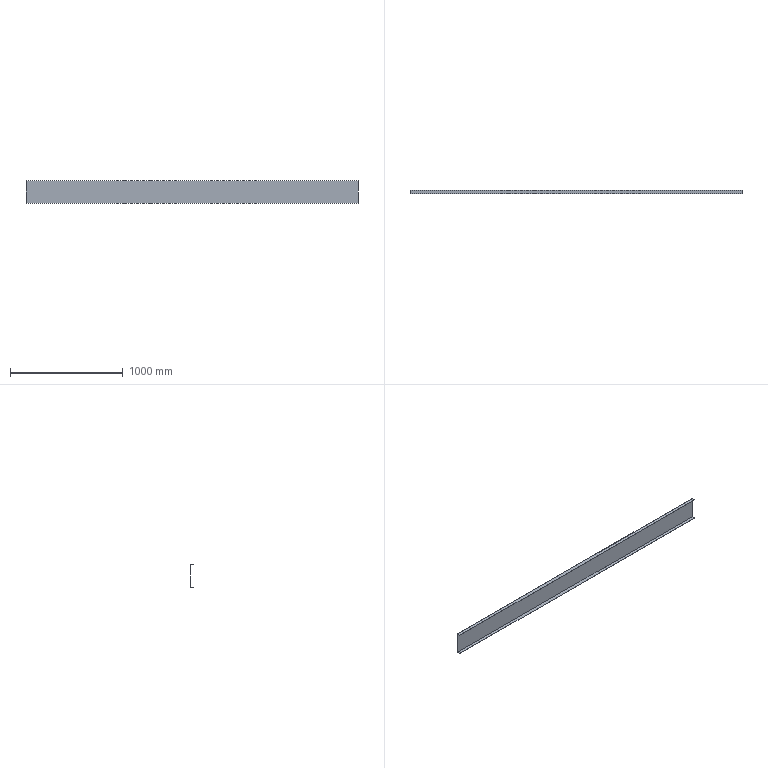Part | STEP file | B-BAN2_1-2 | 1 solid | 10 faces | box 2950 x 30 x 200 mm | volume 1137225 mm3 | plane 10
STEP:
#1=CARTESIAN_POINT('',(2450.,30.,-100.));
#2=VERTEX_POINT('',#1);
#3=CARTESIAN_POINT('',(2450.,30.,100.));
#4=VERTEX_POINT('',#3);
#5=CARTESIAN_POINT('',(2450.,30.,0.));
#6=DIRECTION('',(0.,0.,1.));
#7=VECTOR('',#6,1000.);
#8=LINE('',#5,#7);
#9=EDGE_CURVE('',#2,#4,#8,.T.);
#10=ORIENTED_EDGE('',*,*,#9,.F.);
#11=CARTESIAN_POINT('',(-500.,30.,-100.));
#12=VERTEX_POINT('',#11);
#13=CARTESIAN_POINT('',(0.,30.,-100.));
#14=DIRECTION('',(-1.,0.,0.));
#15=VECTOR('',#14,1000.);
#16=LINE('',#13,#15);
#17=EDGE_CURVE('',#2,#12,#16,.T.);
#18=ORIENTED_EDGE('',*,*,#17,.T.);
#19=CARTESIAN_POINT('',(-500.,30.,100.));
#20=VERTEX_POINT('',#19);
#21=CARTESIAN_POINT('',(-500.,30.,0.));
#22=DIRECTION('',(0.,0.,1.));
#23=VECTOR('',#22,1000.);
#24=LINE('',#21,#23);
#25=EDGE_CURVE('',#12,#20,#24,.T.);
#26=ORIENTED_EDGE('',*,*,#25,.T.);
#27=CARTESIAN_POINT('',(0.,30.,100.));
#28=DIRECTION('',(1.,0.,0.));
#29=VECTOR('',#28,1000.);
#30=LINE('',#27,#29);
#31=EDGE_CURVE('',#20,#4,#30,.T.);
#32=ORIENTED_EDGE('',*,*,#31,.T.);
#33=EDGE_LOOP('',(#10,#18,#26,#32));
#34=FACE_OUTER_BOUND('',#33,.T.);
#35=CARTESIAN_POINT('',(0.,30.,0.));
#36=DIRECTION('',(0.,1.,0.));
#37=DIRECTION('',(0.,0.,1.));
#38=AXIS2_PLACEMENT_3D('',#35,#36,#37);
#39=PLANE('',#38);
#40=ADVANCED_FACE('',(#34),#39,.T.);
#41=CARTESIAN_POINT('',(-500.,0.,-98.5));
#42=VERTEX_POINT('',#41);
#43=CARTESIAN_POINT('',(-500.,28.5,-98.5));
#44=VERTEX_POINT('',#43);
#45=CARTESIAN_POINT('',(-500.,0.,-98.5));
#46=DIRECTION('',(0.,1.,0.));
#47=VECTOR('',#46,1000.);
#48=LINE('',#45,#47);
#49=EDGE_CURVE('',#42,#44,#48,.T.);
#50=ORIENTED_EDGE('',*,*,#49,.T.);
#51=CARTESIAN_POINT('',(-500.,28.5,98.5));
#52=VERTEX_POINT('',#51);
#53=CARTESIAN_POINT('',(-500.,28.5,-100.));
#54=DIRECTION('',(0.,0.,1.));
#55=VECTOR('',#54,1000.);
#56=LINE('',#53,#55);
#57=EDGE_CURVE('',#44,#52,#56,.T.);
#58=ORIENTED_EDGE('',*,*,#57,.T.);
#59=CARTESIAN_POINT('',(-500.,0.,98.5));
#60=VERTEX_POINT('',#59);
#61=CARTESIAN_POINT('',(-500.,0.,98.5));
#62=DIRECTION('',(0.,-1.,0.));
#63=VECTOR('',#62,1000.);
#64=LINE('',#61,#63);
#65=EDGE_CURVE('',#52,#60,#64,.T.);
#66=ORIENTED_EDGE('',*,*,#65,.T.);
#67=CARTESIAN_POINT('',(-500.,0.,100.));
#68=VERTEX_POINT('',#67);
#69=CARTESIAN_POINT('',(-500.,0.,0.));
#70=DIRECTION('',(0.,0.,1.));
#71=VECTOR('',#70,1000.);
#72=LINE('',#69,#71);
#73=EDGE_CURVE('',#60,#68,#72,.T.);
#74=ORIENTED_EDGE('',*,*,#73,.T.);
#75=CARTESIAN_POINT('',(-500.,0.,100.));
#76=DIRECTION('',(0.,1.,0.));
#77=VECTOR('',#76,1000.);
#78=LINE('',#75,#77);
#79=EDGE_CURVE('',#68,#20,#78,.T.);
#80=ORIENTED_EDGE('',*,*,#79,.T.);
#81=ORIENTED_EDGE('',*,*,#25,.F.);
#82=CARTESIAN_POINT('',(-500.,0.,-100.));
#83=VERTEX_POINT('',#82);
#84=CARTESIAN_POINT('',(-500.,0.,-100.));
#85=DIRECTION('',(0.,-1.,0.));
#86=VECTOR('',#85,1000.);
#87=LINE('',#84,#86);
#88=EDGE_CURVE('',#12,#83,#87,.T.);
#89=ORIENTED_EDGE('',*,*,#88,.T.);
#90=CARTESIAN_POINT('',(-500.,0.,0.));
#91=DIRECTION('',(0.,0.,1.));
#92=VECTOR('',#91,1000.);
#93=LINE('',#90,#92);
#94=EDGE_CURVE('',#83,#42,#93,.T.);
#95=ORIENTED_EDGE('',*,*,#94,.T.);
#96=EDGE_LOOP('',(#50,#58,#66,#74,#80,#81,#89,#95));
#97=FACE_OUTER_BOUND('',#96,.T.);
#98=CARTESIAN_POINT('',(-500.,0.,-100.));
#99=DIRECTION('',(-1.,0.,0.));
#100=DIRECTION('',(0.,0.,1.));
#101=AXIS2_PLACEMENT_3D('',#98,#99,#100);
#102=PLANE('',#101);
#103=ADVANCED_FACE('',(#97),#102,.T.);
#104=CARTESIAN_POINT('',(2450.,0.,-100.));
#105=VERTEX_POINT('',#104);
#106=CARTESIAN_POINT('',(2450.,0.,-100.));
#107=DIRECTION('',(0.,1.,0.));
#108=VECTOR('',#107,1000.);
#109=LINE('',#106,#108);
#110=EDGE_CURVE('',#105,#2,#109,.T.);
#111=ORIENTED_EDGE('',*,*,#110,.F.);
#112=CARTESIAN_POINT('',(500.,0.,-100.));
#113=DIRECTION('',(-1.,0.,0.));
#114=VECTOR('',#113,1000.);
#115=LINE('',#112,#114);
#116=EDGE_CURVE('',#105,#83,#115,.T.);
#117=ORIENTED_EDGE('',*,*,#116,.T.);
#118=ORIENTED_EDGE('',*,*,#88,.F.);
#119=ORIENTED_EDGE('',*,*,#17,.F.);
#120=EDGE_LOOP('',(#111,#117,#118,#119));
#121=FACE_OUTER_BOUND('',#120,.T.);
#122=CARTESIAN_POINT('',(500.,0.,-100.));
#123=DIRECTION('',(0.,0.,-1.));
#124=DIRECTION('',(-1.,0.,0.));
#125=AXIS2_PLACEMENT_3D('',#122,#123,#124);
#126=PLANE('',#125);
#127=ADVANCED_FACE('',(#121),#126,.T.);
#128=CARTESIAN_POINT('',(2450.,0.,100.));
#129=VERTEX_POINT('',#128);
#130=CARTESIAN_POINT('',(2450.,0.,100.));
#131=DIRECTION('',(0.,-1.,0.));
#132=VECTOR('',#131,1000.);
#133=LINE('',#130,#132);
#134=EDGE_CURVE('',#4,#129,#133,.T.);
#135=ORIENTED_EDGE('',*,*,#134,.F.);
#136=ORIENTED_EDGE('',*,*,#31,.F.);
#137=ORIENTED_EDGE('',*,*,#79,.F.);
#138=CARTESIAN_POINT('',(-500.,0.,100.));
#139=DIRECTION('',(1.,0.,0.));
#140=VECTOR('',#139,1000.);
#141=LINE('',#138,#140);
#142=EDGE_CURVE('',#68,#129,#141,.T.);
#143=ORIENTED_EDGE('',*,*,#142,.T.);
#144=EDGE_LOOP('',(#135,#136,#137,#143));
#145=FACE_OUTER_BOUND('',#144,.T.);
#146=CARTESIAN_POINT('',(-500.,0.,100.));
#147=DIRECTION('',(0.,0.,1.));
#148=DIRECTION('',(1.,0.,0.));
#149=AXIS2_PLACEMENT_3D('',#146,#147,#148);
#150=PLANE('',#149);
#151=ADVANCED_FACE('',(#145),#150,.T.);
#152=CARTESIAN_POINT('',(2450.,28.5,-98.5));
#153=VERTEX_POINT('',#152);
#154=CARTESIAN_POINT('',(0.,28.5,-98.5));
#155=DIRECTION('',(-1.,0.,0.));
#156=VECTOR('',#155,1000.);
#157=LINE('',#154,#156);
#158=EDGE_CURVE('',#153,#44,#157,.T.);
#159=ORIENTED_EDGE('',*,*,#158,.F.);
#160=CARTESIAN_POINT('',(2450.,28.5,98.5));
#161=VERTEX_POINT('',#160);
#162=CARTESIAN_POINT('',(2450.,28.5,0.));
#163=DIRECTION('',(0.,0.,1.));
#164=VECTOR('',#163,1000.);
#165=LINE('',#162,#164);
#166=EDGE_CURVE('',#153,#161,#165,.T.);
#167=ORIENTED_EDGE('',*,*,#166,.T.);
#168=CARTESIAN_POINT('',(0.,28.5,98.5));
#169=DIRECTION('',(1.,0.,0.));
#170=VECTOR('',#169,1000.);
#171=LINE('',#168,#170);
#172=EDGE_CURVE('',#52,#161,#171,.T.);
#173=ORIENTED_EDGE('',*,*,#172,.F.);
#174=ORIENTED_EDGE('',*,*,#57,.F.);
#175=EDGE_LOOP('',(#159,#167,#173,#174));
#176=FACE_OUTER_BOUND('',#175,.T.);
#177=CARTESIAN_POINT('',(0.,28.5,0.));
#178=DIRECTION('',(0.,1.,0.));
#179=DIRECTION('',(0.,0.,1.));
#180=AXIS2_PLACEMENT_3D('',#177,#178,#179);
#181=PLANE('',#180);
#182=ADVANCED_FACE('',(#176),#181,.F.);
#183=CARTESIAN_POINT('',(2450.,0.,-98.5));
#184=VERTEX_POINT('',#183);
#185=CARTESIAN_POINT('',(500.,0.,-98.5));
#186=DIRECTION('',(-1.,0.,0.));
#187=VECTOR('',#186,1000.);
#188=LINE('',#185,#187);
#189=EDGE_CURVE('',#184,#42,#188,.T.);
#190=ORIENTED_EDGE('',*,*,#189,.F.);
#191=CARTESIAN_POINT('',(2450.,0.,-98.5));
#192=DIRECTION('',(0.,1.,0.));
#193=VECTOR('',#192,1000.);
#194=LINE('',#191,#193);
#195=EDGE_CURVE('',#184,#153,#194,.T.);
#196=ORIENTED_EDGE('',*,*,#195,.T.);
#197=ORIENTED_EDGE('',*,*,#158,.T.);
#198=ORIENTED_EDGE('',*,*,#49,.F.);
#199=EDGE_LOOP('',(#190,#196,#197,#198));
#200=FACE_OUTER_BOUND('',#199,.T.);
#201=CARTESIAN_POINT('',(500.,0.,-98.5));
#202=DIRECTION('',(0.,0.,-1.));
#203=DIRECTION('',(-1.,0.,0.));
#204=AXIS2_PLACEMENT_3D('',#201,#202,#203);
#205=PLANE('',#204);
#206=ADVANCED_FACE('',(#200),#205,.F.);
#207=ORIENTED_EDGE('',*,*,#172,.T.);
#208=CARTESIAN_POINT('',(2450.,0.,98.5));
#209=VERTEX_POINT('',#208);
#210=CARTESIAN_POINT('',(2450.,0.,98.5));
#211=DIRECTION('',(0.,-1.,0.));
#212=VECTOR('',#211,1000.);
#213=LINE('',#210,#212);
#214=EDGE_CURVE('',#161,#209,#213,.T.);
#215=ORIENTED_EDGE('',*,*,#214,.T.);
#216=CARTESIAN_POINT('',(-500.,0.,98.5));
#217=DIRECTION('',(1.,0.,0.));
#218=VECTOR('',#217,1000.);
#219=LINE('',#216,#218);
#220=EDGE_CURVE('',#60,#209,#219,.T.);
#221=ORIENTED_EDGE('',*,*,#220,.F.);
#222=ORIENTED_EDGE('',*,*,#65,.F.);
#223=EDGE_LOOP('',(#207,#215,#221,#222));
#224=FACE_OUTER_BOUND('',#223,.T.);
#225=CARTESIAN_POINT('',(-500.,0.,98.5));
#226=DIRECTION('',(0.,0.,1.));
#227=DIRECTION('',(1.,0.,0.));
#228=AXIS2_PLACEMENT_3D('',#225,#226,#227);
#229=PLANE('',#228);
#230=ADVANCED_FACE('',(#224),#229,.F.);
#231=ORIENTED_EDGE('',*,*,#116,.F.);
#232=CARTESIAN_POINT('',(2450.,0.,175.419));
#233=DIRECTION('',(0.,0.,1.));
#234=VECTOR('',#233,1000.);
#235=LINE('',#232,#234);
#236=EDGE_CURVE('',#105,#184,#235,.T.);
#237=ORIENTED_EDGE('',*,*,#236,.T.);
#238=ORIENTED_EDGE('',*,*,#189,.T.);
#239=ORIENTED_EDGE('',*,*,#94,.F.);
#240=EDGE_LOOP('',(#231,#237,#238,#239));
#241=FACE_OUTER_BOUND('',#240,.T.);
#242=CARTESIAN_POINT('',(0.,0.,0.));
#243=DIRECTION('',(0.,1.,0.));
#244=DIRECTION('',(0.,0.,1.));
#245=AXIS2_PLACEMENT_3D('',#242,#243,#244);
#246=PLANE('',#245);
#247=ADVANCED_FACE('',(#241),#246,.F.);
#248=ORIENTED_EDGE('',*,*,#220,.T.);
#249=CARTESIAN_POINT('',(2450.,0.,175.419));
#250=DIRECTION('',(0.,0.,1.));
#251=VECTOR('',#250,1000.);
#252=LINE('',#249,#251);
#253=EDGE_CURVE('',#209,#129,#252,.T.);
#254=ORIENTED_EDGE('',*,*,#253,.T.);
#255=ORIENTED_EDGE('',*,*,#142,.F.);
#256=ORIENTED_EDGE('',*,*,#73,.F.);
#257=EDGE_LOOP('',(#248,#254,#255,#256));
#258=FACE_OUTER_BOUND('',#257,.T.);
#259=CARTESIAN_POINT('',(0.,0.,0.));
#260=DIRECTION('',(0.,1.,0.));
#261=DIRECTION('',(0.,0.,1.));
#262=AXIS2_PLACEMENT_3D('',#259,#260,#261);
#263=PLANE('',#262);
#264=ADVANCED_FACE('',(#258),#263,.F.);
#265=ORIENTED_EDGE('',*,*,#166,.F.);
#266=ORIENTED_EDGE('',*,*,#195,.F.);
#267=ORIENTED_EDGE('',*,*,#236,.F.);
#268=ORIENTED_EDGE('',*,*,#110,.T.);
#269=ORIENTED_EDGE('',*,*,#9,.T.);
#270=ORIENTED_EDGE('',*,*,#134,.T.);
#271=ORIENTED_EDGE('',*,*,#253,.F.);
#272=ORIENTED_EDGE('',*,*,#214,.F.);
#273=EDGE_LOOP('',(#265,#266,#267,#268,#269,#270,#271,#272));
#274=FACE_OUTER_BOUND('',#273,.T.);
#275=CARTESIAN_POINT('',(2450.,0.,175.419));
#276=DIRECTION('',(-1.,0.,0.));
#277=DIRECTION('',(0.,0.,1.));
#278=AXIS2_PLACEMENT_3D('',#275,#276,#277);
#279=PLANE('',#278);
#280=ADVANCED_FACE('',(#274),#279,.F.);
#281=CLOSED_SHELL('',(#40,#103,#127,#151,#182,#206,#230,#247,#264,#280));
#282=MANIFOLD_SOLID_BREP('',#281);
#283=CARTESIAN_POINT('',(0.,0.,0.));
#284=DIRECTION('',(0.,0.,1.));
#285=DIRECTION('',(1.,0.,0.));
#286=AXIS2_PLACEMENT_3D('',#283,#284,#285);
#287=(LENGTH_UNIT()NAMED_UNIT(*)SI_UNIT(.MILLI.,.METRE.));
#288=UNCERTAINTY_MEASURE_WITH_UNIT(LENGTH_MEASURE(0.00001),#287,'','');
#289=(NAMED_UNIT(*)PLANE_ANGLE_UNIT()SI_UNIT($,.RADIAN.));
#290=(NAMED_UNIT(*)SI_UNIT($,.STERADIAN.)SOLID_ANGLE_UNIT());
#291=(GEOMETRIC_REPRESENTATION_CONTEXT(3)GLOBAL_UNCERTAINTY_ASSIGNED_CONTEXT((#288))GLOBAL_UNIT_ASSIGNED_CONTEXT((#287,#289,#290))REPRESENTATION_CONTEXT('',''));
#292=ADVANCED_BREP_SHAPE_REPRESENTATION('',(#282,#286),#291);